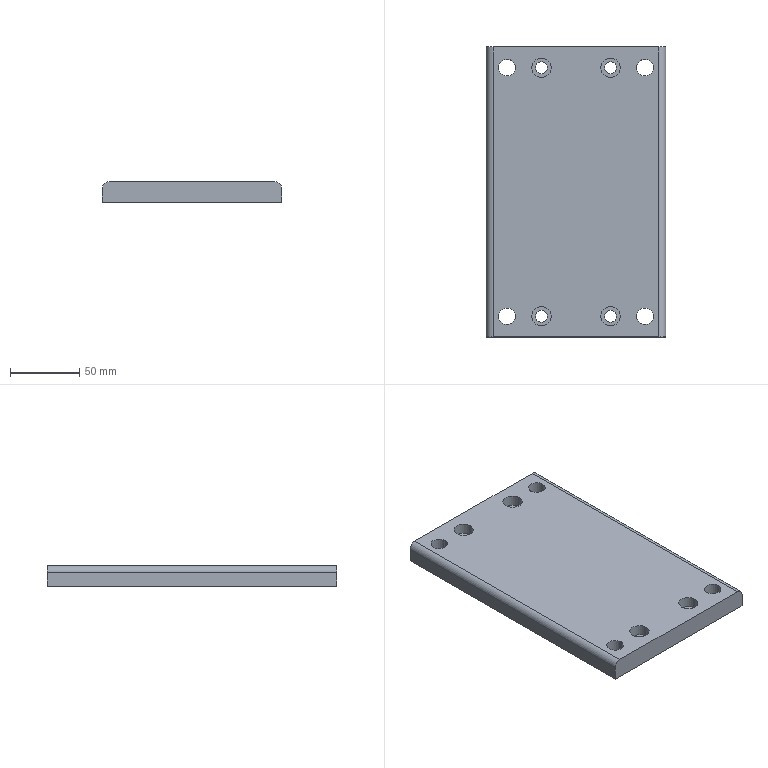Part | STEP file | YBQDJ-YL-3 | 1 solid | 36 faces | box 130 x 210 x 15 mm | volume 393827 mm3 | cylinder 26 | plane 10 | commonest cylinder face diameters 4 x8 1 x4 8.7 x4 12.01 x4 14 x4 10 x2